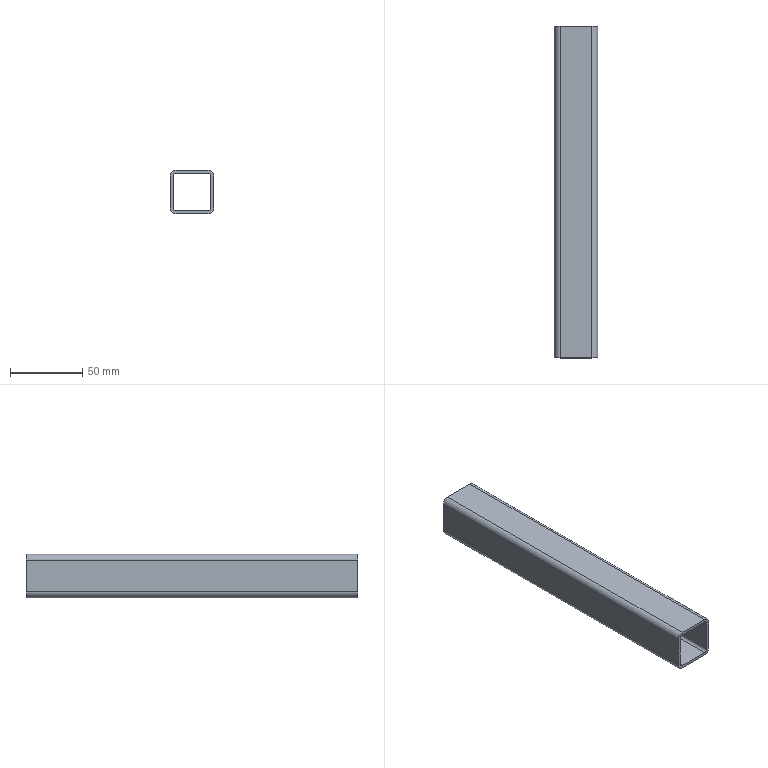Part | SolidWorks | features WeldMemberFeat 1, WeldmentFeature 1 | 1 solid | 18 faces | box 30 x 230 x 30 mm | volume 49151 mm3 | plane 10 | cylinder 8 | commonest cylinder face diameters 4 x4 8 x4
STEP:
#1=CARTESIAN_POINT('',(-15.,0.,11.));
#2=VERTEX_POINT('',#1);
#3=CARTESIAN_POINT('',(-11.,0.,15.));
#4=VERTEX_POINT('',#3);
#5=CARTESIAN_POINT('',(-11.,0.,11.));
#6=DIRECTION('',(0.,1.,0.));
#7=DIRECTION('',(0.,0.,1.));
#8=AXIS2_PLACEMENT_3D('',#5,#6,#7);
#9=CIRCLE('',#8,4.);
#10=EDGE_CURVE('',#2,#4,#9,.T.);
#11=ORIENTED_EDGE('',*,*,#10,.T.);
#12=CARTESIAN_POINT('',(-11.,230.,15.));
#13=VERTEX_POINT('',#12);
#14=CARTESIAN_POINT('',(-11.,230.,15.));
#15=DIRECTION('',(0.,-1.,0.));
#16=VECTOR('',#15,1000.);
#17=LINE('',#14,#16);
#18=EDGE_CURVE('',#13,#4,#17,.T.);
#19=ORIENTED_EDGE('',*,*,#18,.F.);
#20=CARTESIAN_POINT('',(-15.,230.,11.));
#21=VERTEX_POINT('',#20);
#22=CARTESIAN_POINT('',(-11.,230.,11.));
#23=DIRECTION('',(0.,1.,0.));
#24=DIRECTION('',(0.,0.,1.));
#25=AXIS2_PLACEMENT_3D('',#22,#23,#24);
#26=CIRCLE('',#25,4.);
#27=EDGE_CURVE('',#21,#13,#26,.T.);
#28=ORIENTED_EDGE('',*,*,#27,.F.);
#29=CARTESIAN_POINT('',(-15.,230.,11.));
#30=DIRECTION('',(0.,-1.,0.));
#31=VECTOR('',#30,1000.);
#32=LINE('',#29,#31);
#33=EDGE_CURVE('',#21,#2,#32,.T.);
#34=ORIENTED_EDGE('',*,*,#33,.T.);
#35=EDGE_LOOP('',(#11,#19,#28,#34));
#36=FACE_OUTER_BOUND('',#35,.T.);
#37=CARTESIAN_POINT('',(-11.,230.,11.));
#38=DIRECTION('',(0.,-1.,0.));
#39=DIRECTION('',(0.,0.,-1.));
#40=AXIS2_PLACEMENT_3D('',#37,#38,#39);
#41=CYLINDRICAL_SURFACE('',#40,4.);
#42=ADVANCED_FACE('',(#36),#41,.T.);
#43=CARTESIAN_POINT('',(11.,0.,15.));
#44=VERTEX_POINT('',#43);
#45=CARTESIAN_POINT('',(-11.,0.,15.));
#46=DIRECTION('',(1.,0.,0.));
#47=VECTOR('',#46,1000.);
#48=LINE('',#45,#47);
#49=EDGE_CURVE('',#4,#44,#48,.T.);
#50=ORIENTED_EDGE('',*,*,#49,.T.);
#51=CARTESIAN_POINT('',(11.,230.,15.));
#52=VERTEX_POINT('',#51);
#53=CARTESIAN_POINT('',(11.,230.,15.));
#54=DIRECTION('',(0.,-1.,0.));
#55=VECTOR('',#54,1000.);
#56=LINE('',#53,#55);
#57=EDGE_CURVE('',#52,#44,#56,.T.);
#58=ORIENTED_EDGE('',*,*,#57,.F.);
#59=CARTESIAN_POINT('',(-11.,230.,15.));
#60=DIRECTION('',(1.,0.,0.));
#61=VECTOR('',#60,1000.);
#62=LINE('',#59,#61);
#63=EDGE_CURVE('',#13,#52,#62,.T.);
#64=ORIENTED_EDGE('',*,*,#63,.F.);
#65=ORIENTED_EDGE('',*,*,#18,.T.);
#66=EDGE_LOOP('',(#50,#58,#64,#65));
#67=FACE_OUTER_BOUND('',#66,.T.);
#68=CARTESIAN_POINT('',(-11.,230.,15.));
#69=DIRECTION('',(0.,0.,-1.));
#70=DIRECTION('',(-1.,0.,0.));
#71=AXIS2_PLACEMENT_3D('',#68,#69,#70);
#72=PLANE('',#71);
#73=ADVANCED_FACE('',(#67),#72,.F.);
#74=CARTESIAN_POINT('',(15.,0.,11.));
#75=VERTEX_POINT('',#74);
#76=CARTESIAN_POINT('',(11.,0.,11.));
#77=DIRECTION('',(0.,1.,0.));
#78=DIRECTION('',(0.,0.,1.));
#79=AXIS2_PLACEMENT_3D('',#76,#77,#78);
#80=CIRCLE('',#79,4.);
#81=EDGE_CURVE('',#44,#75,#80,.T.);
#82=ORIENTED_EDGE('',*,*,#81,.T.);
#83=CARTESIAN_POINT('',(15.,230.,11.));
#84=VERTEX_POINT('',#83);
#85=CARTESIAN_POINT('',(15.,230.,11.));
#86=DIRECTION('',(0.,-1.,0.));
#87=VECTOR('',#86,1000.);
#88=LINE('',#85,#87);
#89=EDGE_CURVE('',#84,#75,#88,.T.);
#90=ORIENTED_EDGE('',*,*,#89,.F.);
#91=CARTESIAN_POINT('',(11.,230.,11.));
#92=DIRECTION('',(0.,1.,0.));
#93=DIRECTION('',(0.,0.,1.));
#94=AXIS2_PLACEMENT_3D('',#91,#92,#93);
#95=CIRCLE('',#94,4.);
#96=EDGE_CURVE('',#52,#84,#95,.T.);
#97=ORIENTED_EDGE('',*,*,#96,.F.);
#98=ORIENTED_EDGE('',*,*,#57,.T.);
#99=EDGE_LOOP('',(#82,#90,#97,#98));
#100=FACE_OUTER_BOUND('',#99,.T.);
#101=CARTESIAN_POINT('',(11.,230.,11.));
#102=DIRECTION('',(0.,-1.,0.));
#103=DIRECTION('',(0.,0.,-1.));
#104=AXIS2_PLACEMENT_3D('',#101,#102,#103);
#105=CYLINDRICAL_SURFACE('',#104,4.);
#106=ADVANCED_FACE('',(#100),#105,.T.);
#107=CARTESIAN_POINT('',(15.,0.,-11.));
#108=VERTEX_POINT('',#107);
#109=CARTESIAN_POINT('',(15.,0.,-11.));
#110=DIRECTION('',(0.,0.,-1.));
#111=VECTOR('',#110,1000.);
#112=LINE('',#109,#111);
#113=EDGE_CURVE('',#75,#108,#112,.T.);
#114=ORIENTED_EDGE('',*,*,#113,.T.);
#115=CARTESIAN_POINT('',(15.,230.,-11.));
#116=VERTEX_POINT('',#115);
#117=CARTESIAN_POINT('',(15.,230.,-11.));
#118=DIRECTION('',(0.,-1.,0.));
#119=VECTOR('',#118,1000.);
#120=LINE('',#117,#119);
#121=EDGE_CURVE('',#116,#108,#120,.T.);
#122=ORIENTED_EDGE('',*,*,#121,.F.);
#123=CARTESIAN_POINT('',(15.,230.,-11.));
#124=DIRECTION('',(0.,0.,-1.));
#125=VECTOR('',#124,1000.);
#126=LINE('',#123,#125);
#127=EDGE_CURVE('',#84,#116,#126,.T.);
#128=ORIENTED_EDGE('',*,*,#127,.F.);
#129=ORIENTED_EDGE('',*,*,#89,.T.);
#130=EDGE_LOOP('',(#114,#122,#128,#129));
#131=FACE_OUTER_BOUND('',#130,.T.);
#132=CARTESIAN_POINT('',(15.,230.,-11.));
#133=DIRECTION('',(-1.,0.,0.));
#134=DIRECTION('',(0.,0.,1.));
#135=AXIS2_PLACEMENT_3D('',#132,#133,#134);
#136=PLANE('',#135);
#137=ADVANCED_FACE('',(#131),#136,.F.);
#138=CARTESIAN_POINT('',(11.,0.,-15.));
#139=VERTEX_POINT('',#138);
#140=CARTESIAN_POINT('',(11.,0.,-11.));
#141=DIRECTION('',(0.,1.,0.));
#142=DIRECTION('',(0.,0.,1.));
#143=AXIS2_PLACEMENT_3D('',#140,#141,#142);
#144=CIRCLE('',#143,4.);
#145=EDGE_CURVE('',#108,#139,#144,.T.);
#146=ORIENTED_EDGE('',*,*,#145,.T.);
#147=CARTESIAN_POINT('',(11.,230.,-15.));
#148=VERTEX_POINT('',#147);
#149=CARTESIAN_POINT('',(11.,230.,-15.));
#150=DIRECTION('',(0.,-1.,0.));
#151=VECTOR('',#150,1000.);
#152=LINE('',#149,#151);
#153=EDGE_CURVE('',#148,#139,#152,.T.);
#154=ORIENTED_EDGE('',*,*,#153,.F.);
#155=CARTESIAN_POINT('',(11.,230.,-11.));
#156=DIRECTION('',(0.,1.,0.));
#157=DIRECTION('',(0.,0.,1.));
#158=AXIS2_PLACEMENT_3D('',#155,#156,#157);
#159=CIRCLE('',#158,4.);
#160=EDGE_CURVE('',#116,#148,#159,.T.);
#161=ORIENTED_EDGE('',*,*,#160,.F.);
#162=ORIENTED_EDGE('',*,*,#121,.T.);
#163=EDGE_LOOP('',(#146,#154,#161,#162));
#164=FACE_OUTER_BOUND('',#163,.T.);
#165=CARTESIAN_POINT('',(11.,230.,-11.));
#166=DIRECTION('',(0.,-1.,0.));
#167=DIRECTION('',(0.,0.,-1.));
#168=AXIS2_PLACEMENT_3D('',#165,#166,#167);
#169=CYLINDRICAL_SURFACE('',#168,4.);
#170=ADVANCED_FACE('',(#164),#169,.T.);
#171=CARTESIAN_POINT('',(-11.,0.,-15.));
#172=VERTEX_POINT('',#171);
#173=CARTESIAN_POINT('',(11.,0.,-15.));
#174=DIRECTION('',(-1.,0.,0.));
#175=VECTOR('',#174,1000.);
#176=LINE('',#173,#175);
#177=EDGE_CURVE('',#139,#172,#176,.T.);
#178=ORIENTED_EDGE('',*,*,#177,.T.);
#179=CARTESIAN_POINT('',(-11.,230.,-15.));
#180=VERTEX_POINT('',#179);
#181=CARTESIAN_POINT('',(-11.,230.,-15.));
#182=DIRECTION('',(0.,-1.,0.));
#183=VECTOR('',#182,1000.);
#184=LINE('',#181,#183);
#185=EDGE_CURVE('',#180,#172,#184,.T.);
#186=ORIENTED_EDGE('',*,*,#185,.F.);
#187=CARTESIAN_POINT('',(11.,230.,-15.));
#188=DIRECTION('',(-1.,0.,0.));
#189=VECTOR('',#188,1000.);
#190=LINE('',#187,#189);
#191=EDGE_CURVE('',#148,#180,#190,.T.);
#192=ORIENTED_EDGE('',*,*,#191,.F.);
#193=ORIENTED_EDGE('',*,*,#153,.T.);
#194=EDGE_LOOP('',(#178,#186,#192,#193));
#195=FACE_OUTER_BOUND('',#194,.T.);
#196=CARTESIAN_POINT('',(11.,230.,-15.));
#197=DIRECTION('',(0.,0.,1.));
#198=DIRECTION('',(1.,0.,0.));
#199=AXIS2_PLACEMENT_3D('',#196,#197,#198);
#200=PLANE('',#199);
#201=ADVANCED_FACE('',(#195),#200,.F.);
#202=CARTESIAN_POINT('',(-15.,0.,-11.));
#203=VERTEX_POINT('',#202);
#204=CARTESIAN_POINT('',(-11.,0.,-11.));
#205=DIRECTION('',(0.,1.,0.));
#206=DIRECTION('',(0.,0.,1.));
#207=AXIS2_PLACEMENT_3D('',#204,#205,#206);
#208=CIRCLE('',#207,4.);
#209=EDGE_CURVE('',#172,#203,#208,.T.);
#210=ORIENTED_EDGE('',*,*,#209,.T.);
#211=CARTESIAN_POINT('',(-15.,230.,-11.));
#212=VERTEX_POINT('',#211);
#213=CARTESIAN_POINT('',(-15.,230.,-11.));
#214=DIRECTION('',(0.,-1.,0.));
#215=VECTOR('',#214,1000.);
#216=LINE('',#213,#215);
#217=EDGE_CURVE('',#212,#203,#216,.T.);
#218=ORIENTED_EDGE('',*,*,#217,.F.);
#219=CARTESIAN_POINT('',(-11.,230.,-11.));
#220=DIRECTION('',(0.,1.,0.));
#221=DIRECTION('',(0.,0.,1.));
#222=AXIS2_PLACEMENT_3D('',#219,#220,#221);
#223=CIRCLE('',#222,4.);
#224=EDGE_CURVE('',#180,#212,#223,.T.);
#225=ORIENTED_EDGE('',*,*,#224,.F.);
#226=ORIENTED_EDGE('',*,*,#185,.T.);
#227=EDGE_LOOP('',(#210,#218,#225,#226));
#228=FACE_OUTER_BOUND('',#227,.T.);
#229=CARTESIAN_POINT('',(-11.,230.,-11.));
#230=DIRECTION('',(0.,-1.,0.));
#231=DIRECTION('',(0.,0.,-1.));
#232=AXIS2_PLACEMENT_3D('',#229,#230,#231);
#233=CYLINDRICAL_SURFACE('',#232,4.);
#234=ADVANCED_FACE('',(#228),#233,.T.);
#235=CARTESIAN_POINT('',(11.,0.,13.));
#236=VERTEX_POINT('',#235);
#237=CARTESIAN_POINT('',(13.,0.,11.));
#238=VERTEX_POINT('',#237);
#239=CARTESIAN_POINT('',(11.,0.,11.));
#240=DIRECTION('',(0.,1.,0.));
#241=DIRECTION('',(0.,0.,1.));
#242=AXIS2_PLACEMENT_3D('',#239,#240,#241);
#243=CIRCLE('',#242,2.);
#244=EDGE_CURVE('',#236,#238,#243,.T.);
#245=ORIENTED_EDGE('',*,*,#244,.F.);
#246=CARTESIAN_POINT('',(11.,230.,13.));
#247=VERTEX_POINT('',#246);
#248=CARTESIAN_POINT('',(11.,230.,13.));
#249=DIRECTION('',(0.,-1.,0.));
#250=VECTOR('',#249,1000.);
#251=LINE('',#248,#250);
#252=EDGE_CURVE('',#247,#236,#251,.T.);
#253=ORIENTED_EDGE('',*,*,#252,.F.);
#254=CARTESIAN_POINT('',(13.,230.,11.));
#255=VERTEX_POINT('',#254);
#256=CARTESIAN_POINT('',(11.,230.,11.));
#257=DIRECTION('',(0.,1.,0.));
#258=DIRECTION('',(0.,0.,1.));
#259=AXIS2_PLACEMENT_3D('',#256,#257,#258);
#260=CIRCLE('',#259,2.);
#261=EDGE_CURVE('',#247,#255,#260,.T.);
#262=ORIENTED_EDGE('',*,*,#261,.T.);
#263=CARTESIAN_POINT('',(13.,230.,11.));
#264=DIRECTION('',(0.,-1.,0.));
#265=VECTOR('',#264,1000.);
#266=LINE('',#263,#265);
#267=EDGE_CURVE('',#255,#238,#266,.T.);
#268=ORIENTED_EDGE('',*,*,#267,.T.);
#269=EDGE_LOOP('',(#245,#253,#262,#268));
#270=FACE_OUTER_BOUND('',#269,.T.);
#271=CARTESIAN_POINT('',(11.,230.,11.));
#272=DIRECTION('',(0.,-1.,0.));
#273=DIRECTION('',(0.,0.,-1.));
#274=AXIS2_PLACEMENT_3D('',#271,#272,#273);
#275=CYLINDRICAL_SURFACE('',#274,2.);
#276=ADVANCED_FACE('',(#270),#275,.F.);
#277=CARTESIAN_POINT('',(-11.,0.,13.));
#278=VERTEX_POINT('',#277);
#279=CARTESIAN_POINT('',(-11.,0.,13.));
#280=DIRECTION('',(1.,0.,0.));
#281=VECTOR('',#280,1000.);
#282=LINE('',#279,#281);
#283=EDGE_CURVE('',#278,#236,#282,.T.);
#284=ORIENTED_EDGE('',*,*,#283,.F.);
#285=CARTESIAN_POINT('',(-11.,230.,13.));
#286=VERTEX_POINT('',#285);
#287=CARTESIAN_POINT('',(-11.,230.,13.));
#288=DIRECTION('',(0.,-1.,0.));
#289=VECTOR('',#288,1000.);
#290=LINE('',#287,#289);
#291=EDGE_CURVE('',#286,#278,#290,.T.);
#292=ORIENTED_EDGE('',*,*,#291,.F.);
#293=CARTESIAN_POINT('',(-11.,230.,13.));
#294=DIRECTION('',(1.,0.,0.));
#295=VECTOR('',#294,1000.);
#296=LINE('',#293,#295);
#297=EDGE_CURVE('',#286,#247,#296,.T.);
#298=ORIENTED_EDGE('',*,*,#297,.T.);
#299=ORIENTED_EDGE('',*,*,#252,.T.);
#300=EDGE_LOOP('',(#284,#292,#298,#299));
#301=FACE_OUTER_BOUND('',#300,.T.);
#302=CARTESIAN_POINT('',(-11.,230.,13.));
#303=DIRECTION('',(0.,0.,-1.));
#304=DIRECTION('',(-1.,0.,0.));
#305=AXIS2_PLACEMENT_3D('',#302,#303,#304);
#306=PLANE('',#305);
#307=ADVANCED_FACE('',(#301),#306,.T.);
#308=CARTESIAN_POINT('',(-13.,0.,11.));
#309=VERTEX_POINT('',#308);
#310=CARTESIAN_POINT('',(-11.,0.,11.));
#311=DIRECTION('',(0.,1.,0.));
#312=DIRECTION('',(0.,0.,1.));
#313=AXIS2_PLACEMENT_3D('',#310,#311,#312);
#314=CIRCLE('',#313,2.);
#315=EDGE_CURVE('',#309,#278,#314,.T.);
#316=ORIENTED_EDGE('',*,*,#315,.F.);
#317=CARTESIAN_POINT('',(-13.,230.,11.));
#318=VERTEX_POINT('',#317);
#319=CARTESIAN_POINT('',(-13.,230.,11.));
#320=DIRECTION('',(0.,-1.,0.));
#321=VECTOR('',#320,1000.);
#322=LINE('',#319,#321);
#323=EDGE_CURVE('',#318,#309,#322,.T.);
#324=ORIENTED_EDGE('',*,*,#323,.F.);
#325=CARTESIAN_POINT('',(-11.,230.,11.));
#326=DIRECTION('',(0.,1.,0.));
#327=DIRECTION('',(0.,0.,1.));
#328=AXIS2_PLACEMENT_3D('',#325,#326,#327);
#329=CIRCLE('',#328,2.);
#330=EDGE_CURVE('',#318,#286,#329,.T.);
#331=ORIENTED_EDGE('',*,*,#330,.T.);
#332=ORIENTED_EDGE('',*,*,#291,.T.);
#333=EDGE_LOOP('',(#316,#324,#331,#332));
#334=FACE_OUTER_BOUND('',#333,.T.);
#335=CARTESIAN_POINT('',(-11.,230.,11.));
#336=DIRECTION('',(0.,-1.,0.));
#337=DIRECTION('',(0.,0.,-1.));
#338=AXIS2_PLACEMENT_3D('',#335,#336,#337);
#339=CYLINDRICAL_SURFACE('',#338,2.);
#340=ADVANCED_FACE('',(#334),#339,.F.);
#341=CARTESIAN_POINT('',(-13.,0.,-11.));
#342=VERTEX_POINT('',#341);
#343=CARTESIAN_POINT('',(-13.,0.,11.));
#344=DIRECTION('',(0.,0.,1.));
#345=VECTOR('',#344,1000.);
#346=LINE('',#343,#345);
#347=EDGE_CURVE('',#342,#309,#346,.T.);
#348=ORIENTED_EDGE('',*,*,#347,.F.);
#349=CARTESIAN_POINT('',(-13.,230.,-11.));
#350=VERTEX_POINT('',#349);
#351=CARTESIAN_POINT('',(-13.,230.,-11.));
#352=DIRECTION('',(0.,-1.,0.));
#353=VECTOR('',#352,1000.);
#354=LINE('',#351,#353);
#355=EDGE_CURVE('',#350,#342,#354,.T.);
#356=ORIENTED_EDGE('',*,*,#355,.F.);
#357=CARTESIAN_POINT('',(-13.,230.,11.));
#358=DIRECTION('',(0.,0.,1.));
#359=VECTOR('',#358,1000.);
#360=LINE('',#357,#359);
#361=EDGE_CURVE('',#350,#318,#360,.T.);
#362=ORIENTED_EDGE('',*,*,#361,.T.);
#363=ORIENTED_EDGE('',*,*,#323,.T.);
#364=EDGE_LOOP('',(#348,#356,#362,#363));
#365=FACE_OUTER_BOUND('',#364,.T.);
#366=CARTESIAN_POINT('',(-13.,230.,11.));
#367=DIRECTION('',(1.,0.,0.));
#368=DIRECTION('',(0.,0.,-1.));
#369=AXIS2_PLACEMENT_3D('',#366,#367,#368);
#370=PLANE('',#369);
#371=ADVANCED_FACE('',(#365),#370,.T.);
#372=CARTESIAN_POINT('',(-11.,0.,-13.));
#373=VERTEX_POINT('',#372);
#374=CARTESIAN_POINT('',(-11.,0.,-11.));
#375=DIRECTION('',(0.,1.,0.));
#376=DIRECTION('',(0.,0.,1.));
#377=AXIS2_PLACEMENT_3D('',#374,#375,#376);
#378=CIRCLE('',#377,2.);
#379=EDGE_CURVE('',#373,#342,#378,.T.);
#380=ORIENTED_EDGE('',*,*,#379,.F.);
#381=CARTESIAN_POINT('',(-11.,230.,-13.));
#382=VERTEX_POINT('',#381);
#383=CARTESIAN_POINT('',(-11.,230.,-13.));
#384=DIRECTION('',(0.,-1.,0.));
#385=VECTOR('',#384,1000.);
#386=LINE('',#383,#385);
#387=EDGE_CURVE('',#382,#373,#386,.T.);
#388=ORIENTED_EDGE('',*,*,#387,.F.);
#389=CARTESIAN_POINT('',(-11.,230.,-11.));
#390=DIRECTION('',(0.,1.,0.));
#391=DIRECTION('',(0.,0.,1.));
#392=AXIS2_PLACEMENT_3D('',#389,#390,#391);
#393=CIRCLE('',#392,2.);
#394=EDGE_CURVE('',#382,#350,#393,.T.);
#395=ORIENTED_EDGE('',*,*,#394,.T.);
#396=ORIENTED_EDGE('',*,*,#355,.T.);
#397=EDGE_LOOP('',(#380,#388,#395,#396));
#398=FACE_OUTER_BOUND('',#397,.T.);
#399=CARTESIAN_POINT('',(-11.,230.,-11.));
#400=DIRECTION('',(0.,-1.,0.));
#401=DIRECTION('',(0.,0.,-1.));
#402=AXIS2_PLACEMENT_3D('',#399,#400,#401);
#403=CYLINDRICAL_SURFACE('',#402,2.);
#404=ADVANCED_FACE('',(#398),#403,.F.);
#405=CARTESIAN_POINT('',(11.,0.,-13.));
#406=VERTEX_POINT('',#405);
#407=CARTESIAN_POINT('',(11.,0.,-13.));
#408=DIRECTION('',(-1.,0.,0.));
#409=VECTOR('',#408,1000.);
#410=LINE('',#407,#409);
#411=EDGE_CURVE('',#406,#373,#410,.T.);
#412=ORIENTED_EDGE('',*,*,#411,.F.);
#413=CARTESIAN_POINT('',(11.,230.,-13.));
#414=VERTEX_POINT('',#413);
#415=CARTESIAN_POINT('',(11.,230.,-13.));
#416=DIRECTION('',(0.,-1.,0.));
#417=VECTOR('',#416,1000.);
#418=LINE('',#415,#417);
#419=EDGE_CURVE('',#414,#406,#418,.T.);
#420=ORIENTED_EDGE('',*,*,#419,.F.);
#421=CARTESIAN_POINT('',(11.,230.,-13.));
#422=DIRECTION('',(-1.,0.,0.));
#423=VECTOR('',#422,1000.);
#424=LINE('',#421,#423);
#425=EDGE_CURVE('',#414,#382,#424,.T.);
#426=ORIENTED_EDGE('',*,*,#425,.T.);
#427=ORIENTED_EDGE('',*,*,#387,.T.);
#428=EDGE_LOOP('',(#412,#420,#426,#427));
#429=FACE_OUTER_BOUND('',#428,.T.);
#430=CARTESIAN_POINT('',(11.,230.,-13.));
#431=DIRECTION('',(0.,0.,1.));
#432=DIRECTION('',(1.,0.,0.));
#433=AXIS2_PLACEMENT_3D('',#430,#431,#432);
#434=PLANE('',#433);
#435=ADVANCED_FACE('',(#429),#434,.T.);
#436=CARTESIAN_POINT('',(13.,0.,-11.));
#437=VERTEX_POINT('',#436);
#438=CARTESIAN_POINT('',(11.,0.,-11.));
#439=DIRECTION('',(0.,1.,0.));
#440=DIRECTION('',(0.,0.,1.));
#441=AXIS2_PLACEMENT_3D('',#438,#439,#440);
#442=CIRCLE('',#441,2.);
#443=EDGE_CURVE('',#437,#406,#442,.T.);
#444=ORIENTED_EDGE('',*,*,#443,.F.);
#445=CARTESIAN_POINT('',(13.,230.,-11.));
#446=VERTEX_POINT('',#445);
#447=CARTESIAN_POINT('',(13.,230.,-11.));
#448=DIRECTION('',(0.,-1.,0.));
#449=VECTOR('',#448,1000.);
#450=LINE('',#447,#449);
#451=EDGE_CURVE('',#446,#437,#450,.T.);
#452=ORIENTED_EDGE('',*,*,#451,.F.);
#453=CARTESIAN_POINT('',(11.,230.,-11.));
#454=DIRECTION('',(0.,1.,0.));
#455=DIRECTION('',(0.,0.,1.));
#456=AXIS2_PLACEMENT_3D('',#453,#454,#455);
#457=CIRCLE('',#456,2.);
#458=EDGE_CURVE('',#446,#414,#457,.T.);
#459=ORIENTED_EDGE('',*,*,#458,.T.);
#460=ORIENTED_EDGE('',*,*,#419,.T.);
#461=EDGE_LOOP('',(#444,#452,#459,#460));
#462=FACE_OUTER_BOUND('',#461,.T.);
#463=CARTESIAN_POINT('',(11.,230.,-11.));
#464=DIRECTION('',(0.,-1.,0.));
#465=DIRECTION('',(0.,0.,-1.));
#466=AXIS2_PLACEMENT_3D('',#463,#464,#465);
#467=CYLINDRICAL_SURFACE('',#466,2.);
#468=ADVANCED_FACE('',(#462),#467,.F.);
#469=CARTESIAN_POINT('',(13.,0.,-11.));
#470=DIRECTION('',(0.,0.,-1.));
#471=VECTOR('',#470,1000.);
#472=LINE('',#469,#471);
#473=EDGE_CURVE('',#238,#437,#472,.T.);
#474=ORIENTED_EDGE('',*,*,#473,.F.);
#475=ORIENTED_EDGE('',*,*,#267,.F.);
#476=CARTESIAN_POINT('',(13.,230.,-11.));
#477=DIRECTION('',(0.,0.,-1.));
#478=VECTOR('',#477,1000.);
#479=LINE('',#476,#478);
#480=EDGE_CURVE('',#255,#446,#479,.T.);
#481=ORIENTED_EDGE('',*,*,#480,.T.);
#482=ORIENTED_EDGE('',*,*,#451,.T.);
#483=EDGE_LOOP('',(#474,#475,#481,#482));
#484=FACE_OUTER_BOUND('',#483,.T.);
#485=CARTESIAN_POINT('',(13.,230.,-11.));
#486=DIRECTION('',(-1.,0.,0.));
#487=DIRECTION('',(0.,0.,1.));
#488=AXIS2_PLACEMENT_3D('',#485,#486,#487);
#489=PLANE('',#488);
#490=ADVANCED_FACE('',(#484),#489,.T.);
#491=CARTESIAN_POINT('',(-15.,0.,11.));
#492=DIRECTION('',(0.,0.,1.));
#493=VECTOR('',#492,1000.);
#494=LINE('',#491,#493);
#495=EDGE_CURVE('',#203,#2,#494,.T.);
#496=ORIENTED_EDGE('',*,*,#495,.T.);
#497=ORIENTED_EDGE('',*,*,#33,.F.);
#498=CARTESIAN_POINT('',(-15.,230.,11.));
#499=DIRECTION('',(0.,0.,1.));
#500=VECTOR('',#499,1000.);
#501=LINE('',#498,#500);
#502=EDGE_CURVE('',#212,#21,#501,.T.);
#503=ORIENTED_EDGE('',*,*,#502,.F.);
#504=ORIENTED_EDGE('',*,*,#217,.T.);
#505=EDGE_LOOP('',(#496,#497,#503,#504));
#506=FACE_OUTER_BOUND('',#505,.T.);
#507=CARTESIAN_POINT('',(-15.,230.,11.));
#508=DIRECTION('',(1.,0.,0.));
#509=DIRECTION('',(0.,0.,-1.));
#510=AXIS2_PLACEMENT_3D('',#507,#508,#509);
#511=PLANE('',#510);
#512=ADVANCED_FACE('',(#506),#511,.F.);
#513=ORIENTED_EDGE('',*,*,#261,.F.);
#514=ORIENTED_EDGE('',*,*,#297,.F.);
#515=ORIENTED_EDGE('',*,*,#330,.F.);
#516=ORIENTED_EDGE('',*,*,#361,.F.);
#517=ORIENTED_EDGE('',*,*,#394,.F.);
#518=ORIENTED_EDGE('',*,*,#425,.F.);
#519=ORIENTED_EDGE('',*,*,#458,.F.);
#520=ORIENTED_EDGE('',*,*,#480,.F.);
#521=EDGE_LOOP('',(#513,#514,#515,#516,#517,#518,#519,#520));
#522=FACE_BOUND('',#521,.T.);
#523=ORIENTED_EDGE('',*,*,#27,.T.);
#524=ORIENTED_EDGE('',*,*,#63,.T.);
#525=ORIENTED_EDGE('',*,*,#96,.T.);
#526=ORIENTED_EDGE('',*,*,#127,.T.);
#527=ORIENTED_EDGE('',*,*,#160,.T.);
#528=ORIENTED_EDGE('',*,*,#191,.T.);
#529=ORIENTED_EDGE('',*,*,#224,.T.);
#530=ORIENTED_EDGE('',*,*,#502,.T.);
#531=EDGE_LOOP('',(#523,#524,#525,#526,#527,#528,#529,#530));
#532=FACE_OUTER_BOUND('',#531,.T.);
#533=CARTESIAN_POINT('',(-11.,230.,11.));
#534=DIRECTION('',(0.,1.,0.));
#535=DIRECTION('',(0.,0.,1.));
#536=AXIS2_PLACEMENT_3D('',#533,#534,#535);
#537=PLANE('',#536);
#538=ADVANCED_FACE('',(#522,#532),#537,.T.);
#539=ORIENTED_EDGE('',*,*,#244,.T.);
#540=ORIENTED_EDGE('',*,*,#473,.T.);
#541=ORIENTED_EDGE('',*,*,#443,.T.);
#542=ORIENTED_EDGE('',*,*,#411,.T.);
#543=ORIENTED_EDGE('',*,*,#379,.T.);
#544=ORIENTED_EDGE('',*,*,#347,.T.);
#545=ORIENTED_EDGE('',*,*,#315,.T.);
#546=ORIENTED_EDGE('',*,*,#283,.T.);
#547=EDGE_LOOP('',(#539,#540,#541,#542,#543,#544,#545,#546));
#548=FACE_BOUND('',#547,.T.);
#549=ORIENTED_EDGE('',*,*,#10,.F.);
#550=ORIENTED_EDGE('',*,*,#495,.F.);
#551=ORIENTED_EDGE('',*,*,#209,.F.);
#552=ORIENTED_EDGE('',*,*,#177,.F.);
#553=ORIENTED_EDGE('',*,*,#145,.F.);
#554=ORIENTED_EDGE('',*,*,#113,.F.);
#555=ORIENTED_EDGE('',*,*,#81,.F.);
#556=ORIENTED_EDGE('',*,*,#49,.F.);
#557=EDGE_LOOP('',(#549,#550,#551,#552,#553,#554,#555,#556));
#558=FACE_OUTER_BOUND('',#557,.T.);
#559=CARTESIAN_POINT('',(-11.,0.,11.));
#560=DIRECTION('',(0.,1.,0.));
#561=DIRECTION('',(0.,0.,1.));
#562=AXIS2_PLACEMENT_3D('',#559,#560,#561);
#563=PLANE('',#562);
#564=ADVANCED_FACE('',(#548,#558),#563,.F.);
#565=CLOSED_SHELL('',(#42,#73,#106,#137,#170,#201,#234,#276,#307,#340,#371,#404,#435,#468,#490,#512,#538,#564));
#566=MANIFOLD_SOLID_BREP('',#565);
#567=CARTESIAN_POINT('',(0.,0.,0.));
#568=DIRECTION('',(0.,0.,1.));
#569=DIRECTION('',(1.,0.,0.));
#570=AXIS2_PLACEMENT_3D('',#567,#568,#569);
#571=(LENGTH_UNIT()NAMED_UNIT(*)SI_UNIT(.MILLI.,.METRE.));
#572=UNCERTAINTY_MEASURE_WITH_UNIT(LENGTH_MEASURE(0.00001),#571,'','');
#573=(NAMED_UNIT(*)PLANE_ANGLE_UNIT()SI_UNIT($,.RADIAN.));
#574=(NAMED_UNIT(*)SI_UNIT($,.STERADIAN.)SOLID_ANGLE_UNIT());
#575=(GEOMETRIC_REPRESENTATION_CONTEXT(3)GLOBAL_UNCERTAINTY_ASSIGNED_CONTEXT((#572))GLOBAL_UNIT_ASSIGNED_CONTEXT((#571,#573,#574))REPRESENTATION_CONTEXT('',''));
#576=ADVANCED_BREP_SHAPE_REPRESENTATION('',(#566,#570),#575);